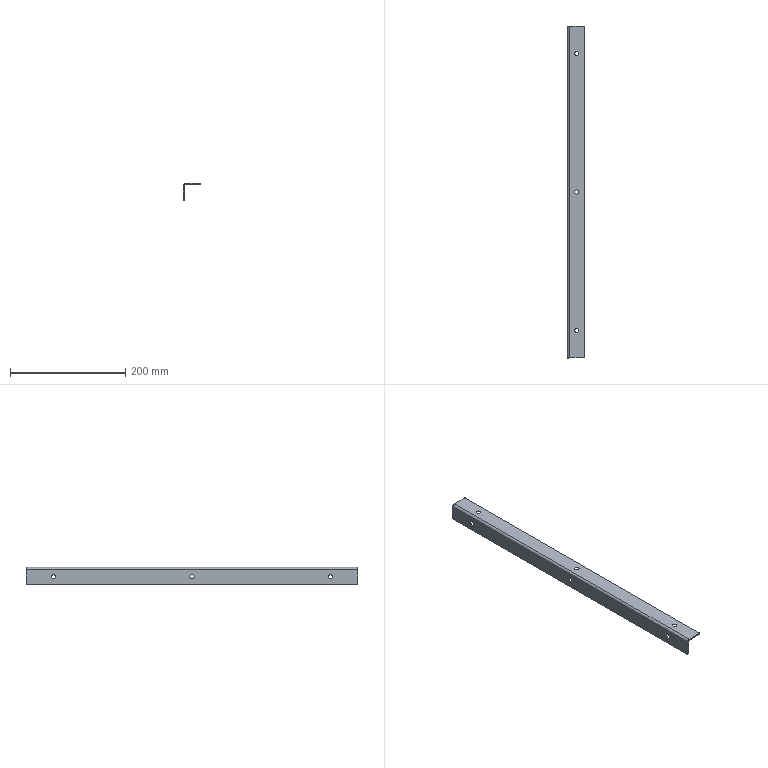Part | SolidWorks | features 3DProfileFeature 2, Fillet 2, HoleWzd 2, FlatPattern 1, ICE 1, LPattern 1, SMBaseFlange 1, SheetMetal 1 | 1 solid | 30 faces | box 30 x 575 x 30 mm | volume 64402 mm3 | cone 12 | plane 12 | cylinder 6 | commonest cylinder face diameters 4 x5 8 x1
STEP:
#1=CARTESIAN_POINT('',(-2.,-245.,-10.4));
#2=VERTEX_POINT('',#1);
#3=CARTESIAN_POINT('',(-2.,-245.,-17.6));
#4=VERTEX_POINT('',#3);
#5=CARTESIAN_POINT('',(-2.,-245.,-14.));
#6=DIRECTION('',(1.,0.,0.));
#7=DIRECTION('',(0.,0.,-1.));
#8=AXIS2_PLACEMENT_3D('',#5,#6,#7);
#9=CIRCLE('',#8,3.6);
#10=EDGE_CURVE('',#2,#4,#9,.T.);
#11=ORIENTED_EDGE('',*,*,#10,.F.);
#12=CARTESIAN_POINT('',(0.,-245.,-8.4));
#13=VERTEX_POINT('',#12);
#14=CARTESIAN_POINT('',(0.,-245.,-8.4));
#15=DIRECTION('',(0.7071,0.,0.7071));
#16=VECTOR('',#15,1000.);
#17=LINE('',#14,#16);
#18=EDGE_CURVE('',#2,#13,#17,.T.);
#19=ORIENTED_EDGE('',*,*,#18,.T.);
#20=CARTESIAN_POINT('',(0.,-245.,-19.6));
#21=VERTEX_POINT('',#20);
#22=CARTESIAN_POINT('',(0.,-245.,-14.));
#23=DIRECTION('',(1.,0.,0.));
#24=DIRECTION('',(0.,0.,-1.));
#25=AXIS2_PLACEMENT_3D('',#22,#23,#24);
#26=CIRCLE('',#25,5.6);
#27=EDGE_CURVE('',#13,#21,#26,.T.);
#28=ORIENTED_EDGE('',*,*,#27,.T.);
#29=CARTESIAN_POINT('',(0.,-245.,-19.6));
#30=DIRECTION('',(0.7071,0.,-0.7071));
#31=VECTOR('',#30,1000.);
#32=LINE('',#29,#31);
#33=EDGE_CURVE('',#4,#21,#32,.T.);
#34=ORIENTED_EDGE('',*,*,#33,.F.);
#35=EDGE_LOOP('',(#11,#19,#28,#34));
#36=FACE_OUTER_BOUND('',#35,.T.);
#37=CARTESIAN_POINT('',(0.,-245.,-14.));
#38=DIRECTION('',(1.,0.,0.));
#39=DIRECTION('',(0.,0.,-1.));
#40=AXIS2_PLACEMENT_3D('',#37,#38,#39);
#41=CONICAL_SURFACE('',#40,5.6,0.7854);
#42=ADVANCED_FACE('',(#36),#41,.F.);
#43=CARTESIAN_POINT('',(-2.,-5.,-10.4));
#44=VERTEX_POINT('',#43);
#45=CARTESIAN_POINT('',(-2.,-5.,-17.6));
#46=VERTEX_POINT('',#45);
#47=CARTESIAN_POINT('',(-2.,-5.,-14.));
#48=DIRECTION('',(1.,0.,0.));
#49=DIRECTION('',(0.,0.,-1.));
#50=AXIS2_PLACEMENT_3D('',#47,#48,#49);
#51=CIRCLE('',#50,3.6);
#52=EDGE_CURVE('',#44,#46,#51,.T.);
#53=ORIENTED_EDGE('',*,*,#52,.F.);
#54=CARTESIAN_POINT('',(0.,-5.,-8.4));
#55=VERTEX_POINT('',#54);
#56=CARTESIAN_POINT('',(0.,-5.,-8.4));
#57=DIRECTION('',(0.7071,0.,0.7071));
#58=VECTOR('',#57,1000.);
#59=LINE('',#56,#58);
#60=EDGE_CURVE('',#44,#55,#59,.T.);
#61=ORIENTED_EDGE('',*,*,#60,.T.);
#62=CARTESIAN_POINT('',(0.,-5.,-19.6));
#63=VERTEX_POINT('',#62);
#64=CARTESIAN_POINT('',(0.,-5.,-14.));
#65=DIRECTION('',(1.,0.,0.));
#66=DIRECTION('',(0.,0.,-1.));
#67=AXIS2_PLACEMENT_3D('',#64,#65,#66);
#68=CIRCLE('',#67,5.6);
#69=EDGE_CURVE('',#55,#63,#68,.T.);
#70=ORIENTED_EDGE('',*,*,#69,.T.);
#71=CARTESIAN_POINT('',(0.,-5.,-19.6));
#72=DIRECTION('',(0.7071,0.,-0.7071));
#73=VECTOR('',#72,1000.);
#74=LINE('',#71,#73);
#75=EDGE_CURVE('',#46,#63,#74,.T.);
#76=ORIENTED_EDGE('',*,*,#75,.F.);
#77=EDGE_LOOP('',(#53,#61,#70,#76));
#78=FACE_OUTER_BOUND('',#77,.T.);
#79=CARTESIAN_POINT('',(0.,-5.,-14.));
#80=DIRECTION('',(1.,0.,0.));
#81=DIRECTION('',(0.,0.,-1.));
#82=AXIS2_PLACEMENT_3D('',#79,#80,#81);
#83=CONICAL_SURFACE('',#82,5.6,0.7854);
#84=ADVANCED_FACE('',(#78),#83,.F.);
#85=CARTESIAN_POINT('',(17.6,-245.,2.));
#86=VERTEX_POINT('',#85);
#87=CARTESIAN_POINT('',(10.4,-245.,2.));
#88=VERTEX_POINT('',#87);
#89=CARTESIAN_POINT('',(14.,-245.,2.));
#90=DIRECTION('',(0.,0.,-1.));
#91=DIRECTION('',(-1.,0.,0.));
#92=AXIS2_PLACEMENT_3D('',#89,#90,#91);
#93=CIRCLE('',#92,3.6);
#94=EDGE_CURVE('',#86,#88,#93,.T.);
#95=ORIENTED_EDGE('',*,*,#94,.F.);
#96=CARTESIAN_POINT('',(19.6,-245.,0.));
#97=VERTEX_POINT('',#96);
#98=CARTESIAN_POINT('',(19.6,-245.,0.));
#99=DIRECTION('',(0.7071,0.,-0.7071));
#100=VECTOR('',#99,1000.);
#101=LINE('',#98,#100);
#102=EDGE_CURVE('',#86,#97,#101,.T.);
#103=ORIENTED_EDGE('',*,*,#102,.T.);
#104=CARTESIAN_POINT('',(8.4,-245.,0.));
#105=VERTEX_POINT('',#104);
#106=CARTESIAN_POINT('',(14.,-245.,0.));
#107=DIRECTION('',(0.,0.,-1.));
#108=DIRECTION('',(-1.,0.,0.));
#109=AXIS2_PLACEMENT_3D('',#106,#107,#108);
#110=CIRCLE('',#109,5.6);
#111=EDGE_CURVE('',#97,#105,#110,.T.);
#112=ORIENTED_EDGE('',*,*,#111,.T.);
#113=CARTESIAN_POINT('',(8.4,-245.,0.));
#114=DIRECTION('',(-0.7071,0.,-0.7071));
#115=VECTOR('',#114,1000.);
#116=LINE('',#113,#115);
#117=EDGE_CURVE('',#88,#105,#116,.T.);
#118=ORIENTED_EDGE('',*,*,#117,.F.);
#119=EDGE_LOOP('',(#95,#103,#112,#118));
#120=FACE_OUTER_BOUND('',#119,.T.);
#121=CARTESIAN_POINT('',(14.,-245.,0.));
#122=DIRECTION('',(0.,0.,-1.));
#123=DIRECTION('',(-1.,0.,0.));
#124=AXIS2_PLACEMENT_3D('',#121,#122,#123);
#125=CONICAL_SURFACE('',#124,5.6,0.7854);
#126=ADVANCED_FACE('',(#120),#125,.F.);
#127=CARTESIAN_POINT('',(17.6,-5.,2.));
#128=VERTEX_POINT('',#127);
#129=CARTESIAN_POINT('',(10.4,-5.,2.));
#130=VERTEX_POINT('',#129);
#131=CARTESIAN_POINT('',(14.,-5.,2.));
#132=DIRECTION('',(0.,0.,-1.));
#133=DIRECTION('',(-1.,0.,0.));
#134=AXIS2_PLACEMENT_3D('',#131,#132,#133);
#135=CIRCLE('',#134,3.6);
#136=EDGE_CURVE('',#128,#130,#135,.T.);
#137=ORIENTED_EDGE('',*,*,#136,.F.);
#138=CARTESIAN_POINT('',(19.6,-5.,0.));
#139=VERTEX_POINT('',#138);
#140=CARTESIAN_POINT('',(19.6,-5.,0.));
#141=DIRECTION('',(0.7071,0.,-0.7071));
#142=VECTOR('',#141,1000.);
#143=LINE('',#140,#142);
#144=EDGE_CURVE('',#128,#139,#143,.T.);
#145=ORIENTED_EDGE('',*,*,#144,.T.);
#146=CARTESIAN_POINT('',(8.4,-5.,0.));
#147=VERTEX_POINT('',#146);
#148=CARTESIAN_POINT('',(14.,-5.,0.));
#149=DIRECTION('',(0.,0.,-1.));
#150=DIRECTION('',(-1.,0.,0.));
#151=AXIS2_PLACEMENT_3D('',#148,#149,#150);
#152=CIRCLE('',#151,5.6);
#153=EDGE_CURVE('',#139,#147,#152,.T.);
#154=ORIENTED_EDGE('',*,*,#153,.T.);
#155=CARTESIAN_POINT('',(8.4,-5.,0.));
#156=DIRECTION('',(-0.7071,0.,-0.7071));
#157=VECTOR('',#156,1000.);
#158=LINE('',#155,#157);
#159=EDGE_CURVE('',#130,#147,#158,.T.);
#160=ORIENTED_EDGE('',*,*,#159,.F.);
#161=EDGE_LOOP('',(#137,#145,#154,#160));
#162=FACE_OUTER_BOUND('',#161,.T.);
#163=CARTESIAN_POINT('',(14.,-5.,0.));
#164=DIRECTION('',(0.,0.,-1.));
#165=DIRECTION('',(-1.,0.,0.));
#166=AXIS2_PLACEMENT_3D('',#163,#164,#165);
#167=CONICAL_SURFACE('',#166,5.6,0.7854);
#168=ADVANCED_FACE('',(#162),#167,.F.);
#169=CARTESIAN_POINT('',(-2.,235.,-10.4));
#170=VERTEX_POINT('',#169);
#171=CARTESIAN_POINT('',(-2.,235.,-17.6));
#172=VERTEX_POINT('',#171);
#173=CARTESIAN_POINT('',(-2.,235.,-14.));
#174=DIRECTION('',(1.,0.,0.));
#175=DIRECTION('',(0.,0.,-1.));
#176=AXIS2_PLACEMENT_3D('',#173,#174,#175);
#177=CIRCLE('',#176,3.6);
#178=EDGE_CURVE('',#170,#172,#177,.T.);
#179=ORIENTED_EDGE('',*,*,#178,.F.);
#180=CARTESIAN_POINT('',(0.,235.,-8.4));
#181=VERTEX_POINT('',#180);
#182=CARTESIAN_POINT('',(0.,235.,-8.4));
#183=DIRECTION('',(0.7071,0.,0.7071));
#184=VECTOR('',#183,1000.);
#185=LINE('',#182,#184);
#186=EDGE_CURVE('',#170,#181,#185,.T.);
#187=ORIENTED_EDGE('',*,*,#186,.T.);
#188=CARTESIAN_POINT('',(0.,235.,-19.6));
#189=VERTEX_POINT('',#188);
#190=CARTESIAN_POINT('',(0.,235.,-14.));
#191=DIRECTION('',(1.,0.,0.));
#192=DIRECTION('',(0.,0.,-1.));
#193=AXIS2_PLACEMENT_3D('',#190,#191,#192);
#194=CIRCLE('',#193,5.6);
#195=EDGE_CURVE('',#181,#189,#194,.T.);
#196=ORIENTED_EDGE('',*,*,#195,.T.);
#197=CARTESIAN_POINT('',(0.,235.,-19.6));
#198=DIRECTION('',(0.7071,0.,-0.7071));
#199=VECTOR('',#198,1000.);
#200=LINE('',#197,#199);
#201=EDGE_CURVE('',#172,#189,#200,.T.);
#202=ORIENTED_EDGE('',*,*,#201,.F.);
#203=EDGE_LOOP('',(#179,#187,#196,#202));
#204=FACE_OUTER_BOUND('',#203,.T.);
#205=CARTESIAN_POINT('',(0.,235.,-14.));
#206=DIRECTION('',(1.,0.,0.));
#207=DIRECTION('',(0.,0.,-1.));
#208=AXIS2_PLACEMENT_3D('',#205,#206,#207);
#209=CONICAL_SURFACE('',#208,5.6,0.7854);
#210=ADVANCED_FACE('',(#204),#209,.F.);
#211=CARTESIAN_POINT('',(17.6,235.,2.));
#212=VERTEX_POINT('',#211);
#213=CARTESIAN_POINT('',(10.4,235.,2.));
#214=VERTEX_POINT('',#213);
#215=CARTESIAN_POINT('',(14.,235.,2.));
#216=DIRECTION('',(0.,0.,-1.));
#217=DIRECTION('',(-1.,0.,0.));
#218=AXIS2_PLACEMENT_3D('',#215,#216,#217);
#219=CIRCLE('',#218,3.6);
#220=EDGE_CURVE('',#212,#214,#219,.T.);
#221=ORIENTED_EDGE('',*,*,#220,.F.);
#222=CARTESIAN_POINT('',(19.6,235.,0.));
#223=VERTEX_POINT('',#222);
#224=CARTESIAN_POINT('',(19.6,235.,0.));
#225=DIRECTION('',(0.7071,0.,-0.7071));
#226=VECTOR('',#225,1000.);
#227=LINE('',#224,#226);
#228=EDGE_CURVE('',#212,#223,#227,.T.);
#229=ORIENTED_EDGE('',*,*,#228,.T.);
#230=CARTESIAN_POINT('',(8.4,235.,0.));
#231=VERTEX_POINT('',#230);
#232=CARTESIAN_POINT('',(14.,235.,0.));
#233=DIRECTION('',(0.,0.,-1.));
#234=DIRECTION('',(-1.,0.,0.));
#235=AXIS2_PLACEMENT_3D('',#232,#233,#234);
#236=CIRCLE('',#235,5.6);
#237=EDGE_CURVE('',#223,#231,#236,.T.);
#238=ORIENTED_EDGE('',*,*,#237,.T.);
#239=CARTESIAN_POINT('',(8.4,235.,0.));
#240=DIRECTION('',(-0.7071,0.,-0.7071));
#241=VECTOR('',#240,1000.);
#242=LINE('',#239,#241);
#243=EDGE_CURVE('',#214,#231,#242,.T.);
#244=ORIENTED_EDGE('',*,*,#243,.F.);
#245=EDGE_LOOP('',(#221,#229,#238,#244));
#246=FACE_OUTER_BOUND('',#245,.T.);
#247=CARTESIAN_POINT('',(14.,235.,0.));
#248=DIRECTION('',(0.,0.,-1.));
#249=DIRECTION('',(-1.,0.,0.));
#250=AXIS2_PLACEMENT_3D('',#247,#248,#249);
#251=CONICAL_SURFACE('',#250,5.6,0.7854);
#252=ADVANCED_FACE('',(#246),#251,.F.);
#253=CARTESIAN_POINT('',(0.,282.5,-26.));
#254=VERTEX_POINT('',#253);
#255=CARTESIAN_POINT('',(0.,282.5,-2.));
#256=VERTEX_POINT('',#255);
#257=CARTESIAN_POINT('',(0.,282.5,-28.));
#258=DIRECTION('',(0.,0.,1.));
#259=VECTOR('',#258,1000.);
#260=LINE('',#257,#259);
#261=EDGE_CURVE('',#254,#256,#260,.T.);
#262=ORIENTED_EDGE('',*,*,#261,.F.);
#263=CARTESIAN_POINT('',(-2.,282.5,-26.));
#264=VERTEX_POINT('',#263);
#265=CARTESIAN_POINT('',(28.,282.5,-26.));
#266=DIRECTION('',(-1.,0.,0.));
#267=VECTOR('',#266,1000.);
#268=LINE('',#265,#267);
#269=EDGE_CURVE('',#254,#264,#268,.T.);
#270=ORIENTED_EDGE('',*,*,#269,.T.);
#271=CARTESIAN_POINT('',(-2.,282.5,-2.));
#272=VERTEX_POINT('',#271);
#273=CARTESIAN_POINT('',(-2.,282.5,18.726));
#274=DIRECTION('',(0.,0.,-1.));
#275=VECTOR('',#274,1000.);
#276=LINE('',#273,#275);
#277=EDGE_CURVE('',#272,#264,#276,.T.);
#278=ORIENTED_EDGE('',*,*,#277,.F.);
#279=CARTESIAN_POINT('',(-2.,282.5,-2.));
#280=DIRECTION('',(1.,0.,0.));
#281=VECTOR('',#280,1000.);
#282=LINE('',#279,#281);
#283=EDGE_CURVE('',#272,#256,#282,.T.);
#284=ORIENTED_EDGE('',*,*,#283,.T.);
#285=EDGE_LOOP('',(#262,#270,#278,#284));
#286=FACE_OUTER_BOUND('',#285,.T.);
#287=CARTESIAN_POINT('',(28.,282.5,18.726));
#288=DIRECTION('',(0.,1.,0.));
#289=DIRECTION('',(0.,0.,1.));
#290=AXIS2_PLACEMENT_3D('',#287,#288,#289);
#291=PLANE('',#290);
#292=ADVANCED_FACE('',(#286),#291,.T.);
#293=CARTESIAN_POINT('',(2.,282.5,2.));
#294=VERTEX_POINT('',#293);
#295=CARTESIAN_POINT('',(26.,282.5,2.));
#296=VERTEX_POINT('',#295);
#297=CARTESIAN_POINT('',(0.,282.5,2.));
#298=DIRECTION('',(1.,0.,0.));
#299=VECTOR('',#298,1000.);
#300=LINE('',#297,#299);
#301=EDGE_CURVE('',#294,#296,#300,.T.);
#302=ORIENTED_EDGE('',*,*,#301,.T.);
#303=CARTESIAN_POINT('',(26.,282.5,0.));
#304=VERTEX_POINT('',#303);
#305=CARTESIAN_POINT('',(26.,282.5,18.726));
#306=DIRECTION('',(0.,0.,-1.));
#307=VECTOR('',#306,1000.);
#308=LINE('',#305,#307);
#309=EDGE_CURVE('',#296,#304,#308,.T.);
#310=ORIENTED_EDGE('',*,*,#309,.T.);
#311=CARTESIAN_POINT('',(2.,282.5,0.));
#312=VERTEX_POINT('',#311);
#313=CARTESIAN_POINT('',(0.,282.5,0.));
#314=DIRECTION('',(1.,0.,0.));
#315=VECTOR('',#314,1000.);
#316=LINE('',#313,#315);
#317=EDGE_CURVE('',#312,#304,#316,.T.);
#318=ORIENTED_EDGE('',*,*,#317,.F.);
#319=CARTESIAN_POINT('',(2.,282.5,0.));
#320=DIRECTION('',(0.,0.,1.));
#321=VECTOR('',#320,1000.);
#322=LINE('',#319,#321);
#323=EDGE_CURVE('',#312,#294,#322,.T.);
#324=ORIENTED_EDGE('',*,*,#323,.T.);
#325=EDGE_LOOP('',(#302,#310,#318,#324));
#326=FACE_OUTER_BOUND('',#325,.T.);
#327=CARTESIAN_POINT('',(28.,282.5,18.726));
#328=DIRECTION('',(0.,1.,0.));
#329=DIRECTION('',(0.,0.,1.));
#330=AXIS2_PLACEMENT_3D('',#327,#328,#329);
#331=PLANE('',#330);
#332=ADVANCED_FACE('',(#326),#331,.T.);
#333=CARTESIAN_POINT('',(14.,235.,2.));
#334=DIRECTION('',(0.,0.,-1.));
#335=DIRECTION('',(-1.,0.,0.));
#336=AXIS2_PLACEMENT_3D('',#333,#334,#335);
#337=CIRCLE('',#336,3.6);
#338=EDGE_CURVE('',#214,#212,#337,.T.);
#339=ORIENTED_EDGE('',*,*,#338,.T.);
#340=ORIENTED_EDGE('',*,*,#220,.T.);
#341=EDGE_LOOP('',(#339,#340));
#342=FACE_BOUND('',#341,.T.);
#343=CARTESIAN_POINT('',(14.,-5.,2.));
#344=DIRECTION('',(0.,0.,-1.));
#345=DIRECTION('',(-1.,0.,0.));
#346=AXIS2_PLACEMENT_3D('',#343,#344,#345);
#347=CIRCLE('',#346,3.6);
#348=EDGE_CURVE('',#130,#128,#347,.T.);
#349=ORIENTED_EDGE('',*,*,#348,.T.);
#350=ORIENTED_EDGE('',*,*,#136,.T.);
#351=EDGE_LOOP('',(#349,#350));
#352=FACE_BOUND('',#351,.T.);
#353=CARTESIAN_POINT('',(14.,-245.,2.));
#354=DIRECTION('',(0.,0.,-1.));
#355=DIRECTION('',(-1.,0.,0.));
#356=AXIS2_PLACEMENT_3D('',#353,#354,#355);
#357=CIRCLE('',#356,3.6);
#358=EDGE_CURVE('',#88,#86,#357,.T.);
#359=ORIENTED_EDGE('',*,*,#358,.T.);
#360=ORIENTED_EDGE('',*,*,#94,.T.);
#361=EDGE_LOOP('',(#359,#360));
#362=FACE_BOUND('',#361,.T.);
#363=CARTESIAN_POINT('',(28.,280.5,2.));
#364=VERTEX_POINT('',#363);
#365=CARTESIAN_POINT('',(28.,-290.5,2.));
#366=VERTEX_POINT('',#365);
#367=CARTESIAN_POINT('',(28.,292.5,2.));
#368=DIRECTION('',(0.,-1.,0.));
#369=VECTOR('',#368,1000.);
#370=LINE('',#367,#369);
#371=EDGE_CURVE('',#364,#366,#370,.T.);
#372=ORIENTED_EDGE('',*,*,#371,.F.);
#373=CARTESIAN_POINT('',(26.,280.5,2.));
#374=DIRECTION('',(0.,0.,1.));
#375=DIRECTION('',(-1.,0.,0.));
#376=AXIS2_PLACEMENT_3D('',#373,#374,#375);
#377=CIRCLE('',#376,2.);
#378=EDGE_CURVE('',#364,#296,#377,.T.);
#379=ORIENTED_EDGE('',*,*,#378,.T.);
#380=ORIENTED_EDGE('',*,*,#301,.F.);
#381=CARTESIAN_POINT('',(2.,-292.5,2.));
#382=VERTEX_POINT('',#381);
#383=CARTESIAN_POINT('',(2.,292.5,2.));
#384=DIRECTION('',(0.,-1.,0.));
#385=VECTOR('',#384,1000.);
#386=LINE('',#383,#385);
#387=EDGE_CURVE('',#294,#382,#386,.T.);
#388=ORIENTED_EDGE('',*,*,#387,.T.);
#389=CARTESIAN_POINT('',(26.,-292.5,2.));
#390=VERTEX_POINT('',#389);
#391=CARTESIAN_POINT('',(0.,-292.5,2.));
#392=DIRECTION('',(1.,0.,0.));
#393=VECTOR('',#392,1000.);
#394=LINE('',#391,#393);
#395=EDGE_CURVE('',#382,#390,#394,.T.);
#396=ORIENTED_EDGE('',*,*,#395,.T.);
#397=CARTESIAN_POINT('',(26.,-290.5,2.));
#398=DIRECTION('',(0.,0.,1.));
#399=DIRECTION('',(-1.,0.,0.));
#400=AXIS2_PLACEMENT_3D('',#397,#398,#399);
#401=CIRCLE('',#400,2.);
#402=EDGE_CURVE('',#390,#366,#401,.T.);
#403=ORIENTED_EDGE('',*,*,#402,.T.);
#404=EDGE_LOOP('',(#372,#379,#380,#388,#396,#403));
#405=FACE_OUTER_BOUND('',#404,.T.);
#406=CARTESIAN_POINT('',(0.,292.5,2.));
#407=DIRECTION('',(0.,0.,-1.));
#408=DIRECTION('',(-1.,0.,0.));
#409=AXIS2_PLACEMENT_3D('',#406,#407,#408);
#410=PLANE('',#409);
#411=ADVANCED_FACE('',(#342,#352,#362,#405),#410,.F.);
#412=CARTESIAN_POINT('',(28.,280.5,0.));
#413=VERTEX_POINT('',#412);
#414=CARTESIAN_POINT('',(28.,-290.5,0.));
#415=VERTEX_POINT('',#414);
#416=CARTESIAN_POINT('',(28.,292.5,0.));
#417=DIRECTION('',(0.,-1.,0.));
#418=VECTOR('',#417,1000.);
#419=LINE('',#416,#418);
#420=EDGE_CURVE('',#413,#415,#419,.T.);
#421=ORIENTED_EDGE('',*,*,#420,.F.);
#422=CARTESIAN_POINT('',(28.,280.5,0.));
#423=DIRECTION('',(0.,0.,1.));
#424=VECTOR('',#423,1000.);
#425=LINE('',#422,#424);
#426=EDGE_CURVE('',#413,#364,#425,.T.);
#427=ORIENTED_EDGE('',*,*,#426,.T.);
#428=ORIENTED_EDGE('',*,*,#371,.T.);
#429=CARTESIAN_POINT('',(28.,-290.5,0.));
#430=DIRECTION('',(0.,0.,-1.));
#431=VECTOR('',#430,1000.);
#432=LINE('',#429,#431);
#433=EDGE_CURVE('',#366,#415,#432,.T.);
#434=ORIENTED_EDGE('',*,*,#433,.T.);
#435=EDGE_LOOP('',(#421,#427,#428,#434));
#436=FACE_OUTER_BOUND('',#435,.T.);
#437=CARTESIAN_POINT('',(28.,292.5,0.));
#438=DIRECTION('',(1.,0.,0.));
#439=DIRECTION('',(0.,0.,-1.));
#440=AXIS2_PLACEMENT_3D('',#437,#438,#439);
#441=PLANE('',#440);
#442=ADVANCED_FACE('',(#436),#441,.T.);
#443=CARTESIAN_POINT('',(14.,-245.,0.));
#444=DIRECTION('',(0.,0.,-1.));
#445=DIRECTION('',(-1.,0.,0.));
#446=AXIS2_PLACEMENT_3D('',#443,#444,#445);
#447=CIRCLE('',#446,5.6);
#448=EDGE_CURVE('',#105,#97,#447,.T.);
#449=ORIENTED_EDGE('',*,*,#448,.F.);
#450=ORIENTED_EDGE('',*,*,#111,.F.);
#451=EDGE_LOOP('',(#449,#450));
#452=FACE_BOUND('',#451,.T.);
#453=CARTESIAN_POINT('',(14.,-5.,0.));
#454=DIRECTION('',(0.,0.,-1.));
#455=DIRECTION('',(-1.,0.,0.));
#456=AXIS2_PLACEMENT_3D('',#453,#454,#455);
#457=CIRCLE('',#456,5.6);
#458=EDGE_CURVE('',#147,#139,#457,.T.);
#459=ORIENTED_EDGE('',*,*,#458,.F.);
#460=ORIENTED_EDGE('',*,*,#153,.F.);
#461=EDGE_LOOP('',(#459,#460));
#462=FACE_BOUND('',#461,.T.);
#463=CARTESIAN_POINT('',(14.,235.,0.));
#464=DIRECTION('',(0.,0.,-1.));
#465=DIRECTION('',(-1.,0.,0.));
#466=AXIS2_PLACEMENT_3D('',#463,#464,#465);
#467=CIRCLE('',#466,5.6);
#468=EDGE_CURVE('',#231,#223,#467,.T.);
#469=ORIENTED_EDGE('',*,*,#468,.F.);
#470=ORIENTED_EDGE('',*,*,#237,.F.);
#471=EDGE_LOOP('',(#469,#470));
#472=FACE_BOUND('',#471,.T.);
#473=ORIENTED_EDGE('',*,*,#317,.T.);
#474=CARTESIAN_POINT('',(26.,280.5,0.));
#475=DIRECTION('',(0.,0.,-1.));
#476=DIRECTION('',(-1.,0.,0.));
#477=AXIS2_PLACEMENT_3D('',#474,#475,#476);
#478=CIRCLE('',#477,2.);
#479=EDGE_CURVE('',#304,#413,#478,.T.);
#480=ORIENTED_EDGE('',*,*,#479,.T.);
#481=ORIENTED_EDGE('',*,*,#420,.T.);
#482=CARTESIAN_POINT('',(26.,-292.5,0.));
#483=VERTEX_POINT('',#482);
#484=CARTESIAN_POINT('',(26.,-290.5,0.));
#485=DIRECTION('',(0.,0.,-1.));
#486=DIRECTION('',(-1.,0.,0.));
#487=AXIS2_PLACEMENT_3D('',#484,#485,#486);
#488=CIRCLE('',#487,2.);
#489=EDGE_CURVE('',#415,#483,#488,.T.);
#490=ORIENTED_EDGE('',*,*,#489,.T.);
#491=CARTESIAN_POINT('',(2.,-292.5,0.));
#492=VERTEX_POINT('',#491);
#493=CARTESIAN_POINT('',(0.,-292.5,0.));
#494=DIRECTION('',(1.,0.,0.));
#495=VECTOR('',#494,1000.);
#496=LINE('',#493,#495);
#497=EDGE_CURVE('',#492,#483,#496,.T.);
#498=ORIENTED_EDGE('',*,*,#497,.F.);
#499=CARTESIAN_POINT('',(2.,292.5,0.));
#500=DIRECTION('',(0.,-1.,0.));
#501=VECTOR('',#500,1000.);
#502=LINE('',#499,#501);
#503=EDGE_CURVE('',#312,#492,#502,.T.);
#504=ORIENTED_EDGE('',*,*,#503,.F.);
#505=EDGE_LOOP('',(#473,#480,#481,#490,#498,#504));
#506=FACE_OUTER_BOUND('',#505,.T.);
#507=CARTESIAN_POINT('',(0.,292.5,0.));
#508=DIRECTION('',(0.,0.,-1.));
#509=DIRECTION('',(-1.,0.,0.));
#510=AXIS2_PLACEMENT_3D('',#507,#508,#509);
#511=PLANE('',#510);
#512=ADVANCED_FACE('',(#452,#462,#472,#506),#511,.T.);
#513=CARTESIAN_POINT('',(0.,-292.5,-2.));
#514=VERTEX_POINT('',#513);
#515=CARTESIAN_POINT('',(0.,292.5,-2.));
#516=DIRECTION('',(0.,-1.,0.));
#517=VECTOR('',#516,1000.);
#518=LINE('',#515,#517);
#519=EDGE_CURVE('',#256,#514,#518,.T.);
#520=ORIENTED_EDGE('',*,*,#519,.F.);
#521=CARTESIAN_POINT('',(2.,282.5,-2.));
#522=DIRECTION('',(0.,1.,0.));
#523=DIRECTION('',(0.,0.,1.));
#524=AXIS2_PLACEMENT_3D('',#521,#522,#523);
#525=CIRCLE('',#524,2.);
#526=EDGE_CURVE('',#256,#312,#525,.T.);
#527=ORIENTED_EDGE('',*,*,#526,.T.);
#528=ORIENTED_EDGE('',*,*,#503,.T.);
#529=CARTESIAN_POINT('',(2.,-292.5,-2.));
#530=DIRECTION('',(0.,1.,0.));
#531=DIRECTION('',(0.,0.,-1.));
#532=AXIS2_PLACEMENT_3D('',#529,#530,#531);
#533=CIRCLE('',#532,2.);
#534=EDGE_CURVE('',#514,#492,#533,.T.);
#535=ORIENTED_EDGE('',*,*,#534,.F.);
#536=EDGE_LOOP('',(#520,#527,#528,#535));
#537=FACE_OUTER_BOUND('',#536,.T.);
#538=CARTESIAN_POINT('',(2.,292.5,-2.));
#539=DIRECTION('',(0.,-1.,0.));
#540=DIRECTION('',(0.,0.,-1.));
#541=AXIS2_PLACEMENT_3D('',#538,#539,#540);
#542=CYLINDRICAL_SURFACE('',#541,2.);
#543=ADVANCED_FACE('',(#537),#542,.F.);
#544=CARTESIAN_POINT('',(0.,-245.,-14.));
#545=DIRECTION('',(1.,0.,0.));
#546=DIRECTION('',(0.,0.,-1.));
#547=AXIS2_PLACEMENT_3D('',#544,#545,#546);
#548=CIRCLE('',#547,5.6);
#549=EDGE_CURVE('',#21,#13,#548,.T.);
#550=ORIENTED_EDGE('',*,*,#549,.F.);
#551=ORIENTED_EDGE('',*,*,#27,.F.);
#552=EDGE_LOOP('',(#550,#551));
#553=FACE_BOUND('',#552,.T.);
#554=CARTESIAN_POINT('',(0.,-5.,-14.));
#555=DIRECTION('',(1.,0.,0.));
#556=DIRECTION('',(0.,0.,-1.));
#557=AXIS2_PLACEMENT_3D('',#554,#555,#556);
#558=CIRCLE('',#557,5.6);
#559=EDGE_CURVE('',#63,#55,#558,.T.);
#560=ORIENTED_EDGE('',*,*,#559,.F.);
#561=ORIENTED_EDGE('',*,*,#69,.F.);
#562=EDGE_LOOP('',(#560,#561));
#563=FACE_BOUND('',#562,.T.);
#564=CARTESIAN_POINT('',(0.,235.,-14.));
#565=DIRECTION('',(1.,0.,0.));
#566=DIRECTION('',(0.,0.,-1.));
#567=AXIS2_PLACEMENT_3D('',#564,#565,#566);
#568=CIRCLE('',#567,5.6);
#569=EDGE_CURVE('',#189,#181,#568,.T.);
#570=ORIENTED_EDGE('',*,*,#569,.F.);
#571=ORIENTED_EDGE('',*,*,#195,.F.);
#572=EDGE_LOOP('',(#570,#571));
#573=FACE_BOUND('',#572,.T.);
#574=CARTESIAN_POINT('',(0.,280.5,-28.));
#575=VERTEX_POINT('',#574);
#576=CARTESIAN_POINT('',(0.,-290.5,-28.));
#577=VERTEX_POINT('',#576);
#578=CARTESIAN_POINT('',(0.,292.5,-28.));
#579=DIRECTION('',(0.,-1.,0.));
#580=VECTOR('',#579,1000.);
#581=LINE('',#578,#580);
#582=EDGE_CURVE('',#575,#577,#581,.T.);
#583=ORIENTED_EDGE('',*,*,#582,.F.);
#584=CARTESIAN_POINT('',(0.,280.5,-26.));
#585=DIRECTION('',(1.,0.,0.));
#586=DIRECTION('',(0.,0.,-1.));
#587=AXIS2_PLACEMENT_3D('',#584,#585,#586);
#588=CIRCLE('',#587,2.);
#589=EDGE_CURVE('',#575,#254,#588,.T.);
#590=ORIENTED_EDGE('',*,*,#589,.T.);
#591=ORIENTED_EDGE('',*,*,#261,.T.);
#592=ORIENTED_EDGE('',*,*,#519,.T.);
#593=CARTESIAN_POINT('',(0.,-292.5,-26.));
#594=VERTEX_POINT('',#593);
#595=CARTESIAN_POINT('',(0.,-292.5,-28.));
#596=DIRECTION('',(0.,0.,1.));
#597=VECTOR('',#596,1000.);
#598=LINE('',#595,#597);
#599=EDGE_CURVE('',#594,#514,#598,.T.);
#600=ORIENTED_EDGE('',*,*,#599,.F.);
#601=CARTESIAN_POINT('',(0.,-290.5,-26.));
#602=DIRECTION('',(1.,0.,0.));
#603=DIRECTION('',(0.,0.,-1.));
#604=AXIS2_PLACEMENT_3D('',#601,#602,#603);
#605=CIRCLE('',#604,2.);
#606=EDGE_CURVE('',#594,#577,#605,.T.);
#607=ORIENTED_EDGE('',*,*,#606,.T.);
#608=EDGE_LOOP('',(#583,#590,#591,#592,#600,#607));
#609=FACE_OUTER_BOUND('',#608,.T.);
#610=CARTESIAN_POINT('',(0.,292.5,-28.));
#611=DIRECTION('',(1.,0.,0.));
#612=DIRECTION('',(0.,0.,-1.));
#613=AXIS2_PLACEMENT_3D('',#610,#611,#612);
#614=PLANE('',#613);
#615=ADVANCED_FACE('',(#553,#563,#573,#609),#614,.T.);
#616=CARTESIAN_POINT('',(-2.,280.5,-28.));
#617=VERTEX_POINT('',#616);
#618=CARTESIAN_POINT('',(-2.,-290.5,-28.));
#619=VERTEX_POINT('',#618);
#620=CARTESIAN_POINT('',(-2.,292.5,-28.));
#621=DIRECTION('',(0.,-1.,0.));
#622=VECTOR('',#621,1000.);
#623=LINE('',#620,#622);
#624=EDGE_CURVE('',#617,#619,#623,.T.);
#625=ORIENTED_EDGE('',*,*,#624,.F.);
#626=CARTESIAN_POINT('',(-2.,280.5,-28.));
#627=DIRECTION('',(1.,0.,0.));
#628=VECTOR('',#627,1000.);
#629=LINE('',#626,#628);
#630=EDGE_CURVE('',#617,#575,#629,.T.);
#631=ORIENTED_EDGE('',*,*,#630,.T.);
#632=ORIENTED_EDGE('',*,*,#582,.T.);
#633=CARTESIAN_POINT('',(-2.,-290.5,-28.));
#634=DIRECTION('',(-1.,0.,0.));
#635=VECTOR('',#634,1000.);
#636=LINE('',#633,#635);
#637=EDGE_CURVE('',#577,#619,#636,.T.);
#638=ORIENTED_EDGE('',*,*,#637,.T.);
#639=EDGE_LOOP('',(#625,#631,#632,#638));
#640=FACE_OUTER_BOUND('',#639,.T.);
#641=CARTESIAN_POINT('',(-2.,292.5,-28.));
#642=DIRECTION('',(0.,0.,-1.));
#643=DIRECTION('',(-1.,0.,0.));
#644=AXIS2_PLACEMENT_3D('',#641,#642,#643);
#645=PLANE('',#644);
#646=ADVANCED_FACE('',(#640),#645,.T.);
#647=CARTESIAN_POINT('',(-2.,235.,-14.));
#648=DIRECTION('',(1.,0.,0.));
#649=DIRECTION('',(0.,0.,-1.));
#650=AXIS2_PLACEMENT_3D('',#647,#648,#649);
#651=CIRCLE('',#650,3.6);
#652=EDGE_CURVE('',#172,#170,#651,.T.);
#653=ORIENTED_EDGE('',*,*,#652,.T.);
#654=ORIENTED_EDGE('',*,*,#178,.T.);
#655=EDGE_LOOP('',(#653,#654));
#656=FACE_BOUND('',#655,.T.);
#657=CARTESIAN_POINT('',(-2.,-5.,-14.));
#658=DIRECTION('',(1.,0.,0.));
#659=DIRECTION('',(0.,0.,-1.));
#660=AXIS2_PLACEMENT_3D('',#657,#658,#659);
#661=CIRCLE('',#660,3.6);
#662=EDGE_CURVE('',#46,#44,#661,.T.);
#663=ORIENTED_EDGE('',*,*,#662,.T.);
#664=ORIENTED_EDGE('',*,*,#52,.T.);
#665=EDGE_LOOP('',(#663,#664));
#666=FACE_BOUND('',#665,.T.);
#667=CARTESIAN_POINT('',(-2.,-245.,-14.));
#668=DIRECTION('',(1.,0.,0.));
#669=DIRECTION('',(0.,0.,-1.));
#670=AXIS2_PLACEMENT_3D('',#667,#668,#669);
#671=CIRCLE('',#670,3.6);
#672=EDGE_CURVE('',#4,#2,#671,.T.);
#673=ORIENTED_EDGE('',*,*,#672,.T.);
#674=ORIENTED_EDGE('',*,*,#10,.T.);
#675=EDGE_LOOP('',(#673,#674));
#676=FACE_BOUND('',#675,.T.);
#677=ORIENTED_EDGE('',*,*,#277,.T.);
#678=CARTESIAN_POINT('',(-2.,280.5,-26.));
#679=DIRECTION('',(-1.,0.,0.));
#680=DIRECTION('',(0.,0.,-1.));
#681=AXIS2_PLACEMENT_3D('',#678,#679,#680);
#682=CIRCLE('',#681,2.);
#683=EDGE_CURVE('',#264,#617,#682,.T.);
#684=ORIENTED_EDGE('',*,*,#683,.T.);
#685=ORIENTED_EDGE('',*,*,#624,.T.);
#686=CARTESIAN_POINT('',(-2.,-292.5,-26.));
#687=VERTEX_POINT('',#686);
#688=CARTESIAN_POINT('',(-2.,-290.5,-26.));
#689=DIRECTION('',(-1.,0.,0.));
#690=DIRECTION('',(0.,0.,-1.));
#691=AXIS2_PLACEMENT_3D('',#688,#689,#690);
#692=CIRCLE('',#691,2.);
#693=EDGE_CURVE('',#619,#687,#692,.T.);
#694=ORIENTED_EDGE('',*,*,#693,.T.);
#695=CARTESIAN_POINT('',(-2.,-292.5,-2.));
#696=VERTEX_POINT('',#695);
#697=CARTESIAN_POINT('',(-2.,-292.5,-28.));
#698=DIRECTION('',(0.,0.,1.));
#699=VECTOR('',#698,1000.);
#700=LINE('',#697,#699);
#701=EDGE_CURVE('',#687,#696,#700,.T.);
#702=ORIENTED_EDGE('',*,*,#701,.T.);
#703=CARTESIAN_POINT('',(-2.,292.5,-2.));
#704=DIRECTION('',(0.,-1.,0.));
#705=VECTOR('',#704,1000.);
#706=LINE('',#703,#705);
#707=EDGE_CURVE('',#272,#696,#706,.T.);
#708=ORIENTED_EDGE('',*,*,#707,.F.);
#709=EDGE_LOOP('',(#677,#684,#685,#694,#702,#708));
#710=FACE_OUTER_BOUND('',#709,.T.);
#711=CARTESIAN_POINT('',(-2.,292.5,-28.));
#712=DIRECTION('',(1.,0.,0.));
#713=DIRECTION('',(0.,0.,-1.));
#714=AXIS2_PLACEMENT_3D('',#711,#712,#713);
#715=PLANE('',#714);
#716=ADVANCED_FACE('',(#656,#666,#676,#710),#715,.F.);
#717=CARTESIAN_POINT('',(2.,282.5,-2.));
#718=DIRECTION('',(0.,1.,0.));
#719=DIRECTION('',(0.,0.,1.));
#720=AXIS2_PLACEMENT_3D('',#717,#718,#719);
#721=CIRCLE('',#720,4.);
#722=EDGE_CURVE('',#272,#294,#721,.T.);
#723=ORIENTED_EDGE('',*,*,#722,.F.);
#724=ORIENTED_EDGE('',*,*,#707,.T.);
#725=CARTESIAN_POINT('',(2.,-292.5,-2.));
#726=DIRECTION('',(0.,1.,0.));
#727=DIRECTION('',(1.,0.,0.));
#728=AXIS2_PLACEMENT_3D('',#725,#726,#727);
#729=CIRCLE('',#728,4.);
#730=EDGE_CURVE('',#696,#382,#729,.T.);
#731=ORIENTED_EDGE('',*,*,#730,.T.);
#732=ORIENTED_EDGE('',*,*,#387,.F.);
#733=EDGE_LOOP('',(#723,#724,#731,#732));
#734=FACE_OUTER_BOUND('',#733,.T.);
#735=CARTESIAN_POINT('',(2.,292.5,-2.));
#736=DIRECTION('',(0.,-1.,0.));
#737=DIRECTION('',(0.,0.,-1.));
#738=AXIS2_PLACEMENT_3D('',#735,#736,#737);
#739=CYLINDRICAL_SURFACE('',#738,4.);
#740=ADVANCED_FACE('',(#734),#739,.T.);
#741=CARTESIAN_POINT('',(0.,-292.5,-2.));
#742=DIRECTION('',(-1.,0.,0.));
#743=VECTOR('',#742,1000.);
#744=LINE('',#741,#743);
#745=EDGE_CURVE('',#514,#696,#744,.T.);
#746=ORIENTED_EDGE('',*,*,#745,.F.);
#747=ORIENTED_EDGE('',*,*,#534,.T.);
#748=CARTESIAN_POINT('',(2.,-292.5,2.));
#749=DIRECTION('',(0.,0.,-1.));
#750=VECTOR('',#749,1000.);
#751=LINE('',#748,#750);
#752=EDGE_CURVE('',#382,#492,#751,.T.);
#753=ORIENTED_EDGE('',*,*,#752,.F.);
#754=ORIENTED_EDGE('',*,*,#730,.F.);
#755=EDGE_LOOP('',(#746,#747,#753,#754));
#756=FACE_OUTER_BOUND('',#755,.T.);
#757=CARTESIAN_POINT('',(0.,-292.5,-2.));
#758=DIRECTION('',(0.,-1.,0.));
#759=DIRECTION('',(0.,0.,-1.));
#760=AXIS2_PLACEMENT_3D('',#757,#758,#759);
#761=PLANE('',#760);
#762=ADVANCED_FACE('',(#756),#761,.T.);
#763=ORIENTED_EDGE('',*,*,#701,.F.);
#764=CARTESIAN_POINT('',(2.,-292.5,-26.));
#765=DIRECTION('',(1.,0.,0.));
#766=VECTOR('',#765,1000.);
#767=LINE('',#764,#766);
#768=EDGE_CURVE('',#687,#594,#767,.T.);
#769=ORIENTED_EDGE('',*,*,#768,.T.);
#770=ORIENTED_EDGE('',*,*,#599,.T.);
#771=ORIENTED_EDGE('',*,*,#745,.T.);
#772=EDGE_LOOP('',(#763,#769,#770,#771));
#773=FACE_OUTER_BOUND('',#772,.T.);
#774=CARTESIAN_POINT('',(2.,-292.5,2.));
#775=DIRECTION('',(0.,-1.,0.));
#776=DIRECTION('',(0.,0.,-1.));
#777=AXIS2_PLACEMENT_3D('',#774,#775,#776);
#778=PLANE('',#777);
#779=ADVANCED_FACE('',(#773),#778,.T.);
#780=ORIENTED_EDGE('',*,*,#497,.T.);
#781=CARTESIAN_POINT('',(26.,-292.5,-2.));
#782=DIRECTION('',(0.,0.,1.));
#783=VECTOR('',#782,1000.);
#784=LINE('',#781,#783);
#785=EDGE_CURVE('',#483,#390,#784,.T.);
#786=ORIENTED_EDGE('',*,*,#785,.T.);
#787=ORIENTED_EDGE('',*,*,#395,.F.);
#788=ORIENTED_EDGE('',*,*,#752,.T.);
#789=EDGE_LOOP('',(#780,#786,#787,#788));
#790=FACE_OUTER_BOUND('',#789,.T.);
#791=CARTESIAN_POINT('',(2.,-292.5,-2.));
#792=DIRECTION('',(0.,-1.,0.));
#793=DIRECTION('',(-1.,0.,0.));
#794=AXIS2_PLACEMENT_3D('',#791,#792,#793);
#795=PLANE('',#794);
#796=ADVANCED_FACE('',(#790),#795,.T.);
#797=ORIENTED_EDGE('',*,*,#489,.F.);
#798=ORIENTED_EDGE('',*,*,#433,.F.);
#799=ORIENTED_EDGE('',*,*,#402,.F.);
#800=ORIENTED_EDGE('',*,*,#785,.F.);
#801=EDGE_LOOP('',(#797,#798,#799,#800));
#802=FACE_OUTER_BOUND('',#801,.T.);
#803=CARTESIAN_POINT('',(26.,-290.5,-2.));
#804=DIRECTION('',(0.,0.,1.));
#805=DIRECTION('',(1.,0.,0.));
#806=AXIS2_PLACEMENT_3D('',#803,#804,#805);
#807=CYLINDRICAL_SURFACE('',#806,2.);
#808=ADVANCED_FACE('',(#802),#807,.T.);
#809=ORIENTED_EDGE('',*,*,#693,.F.);
#810=ORIENTED_EDGE('',*,*,#637,.F.);
#811=ORIENTED_EDGE('',*,*,#606,.F.);
#812=ORIENTED_EDGE('',*,*,#768,.F.);
#813=EDGE_LOOP('',(#809,#810,#811,#812));
#814=FACE_OUTER_BOUND('',#813,.T.);
#815=CARTESIAN_POINT('',(2.,-290.5,-26.));
#816=DIRECTION('',(1.,0.,0.));
#817=DIRECTION('',(0.,0.,-1.));
#818=AXIS2_PLACEMENT_3D('',#815,#816,#817);
#819=CYLINDRICAL_SURFACE('',#818,2.);
#820=ADVANCED_FACE('',(#814),#819,.T.);
#821=ORIENTED_EDGE('',*,*,#228,.F.);
#822=ORIENTED_EDGE('',*,*,#338,.F.);
#823=ORIENTED_EDGE('',*,*,#243,.T.);
#824=ORIENTED_EDGE('',*,*,#468,.T.);
#825=EDGE_LOOP('',(#821,#822,#823,#824));
#826=FACE_OUTER_BOUND('',#825,.T.);
#827=CARTESIAN_POINT('',(14.,235.,0.));
#828=DIRECTION('',(0.,0.,-1.));
#829=DIRECTION('',(-1.,0.,0.));
#830=AXIS2_PLACEMENT_3D('',#827,#828,#829);
#831=CONICAL_SURFACE('',#830,5.6,0.7854);
#832=ADVANCED_FACE('',(#826),#831,.F.);
#833=ORIENTED_EDGE('',*,*,#186,.F.);
#834=ORIENTED_EDGE('',*,*,#652,.F.);
#835=ORIENTED_EDGE('',*,*,#201,.T.);
#836=ORIENTED_EDGE('',*,*,#569,.T.);
#837=EDGE_LOOP('',(#833,#834,#835,#836));
#838=FACE_OUTER_BOUND('',#837,.T.);
#839=CARTESIAN_POINT('',(0.,235.,-14.));
#840=DIRECTION('',(1.,0.,0.));
#841=DIRECTION('',(0.,0.,-1.));
#842=AXIS2_PLACEMENT_3D('',#839,#840,#841);
#843=CONICAL_SURFACE('',#842,5.6,0.7854);
#844=ADVANCED_FACE('',(#838),#843,.F.);
#845=ORIENTED_EDGE('',*,*,#144,.F.);
#846=ORIENTED_EDGE('',*,*,#348,.F.);
#847=ORIENTED_EDGE('',*,*,#159,.T.);
#848=ORIENTED_EDGE('',*,*,#458,.T.);
#849=EDGE_LOOP('',(#845,#846,#847,#848));
#850=FACE_OUTER_BOUND('',#849,.T.);
#851=CARTESIAN_POINT('',(14.,-5.,0.));
#852=DIRECTION('',(0.,0.,-1.));
#853=DIRECTION('',(-1.,0.,0.));
#854=AXIS2_PLACEMENT_3D('',#851,#852,#853);
#855=CONICAL_SURFACE('',#854,5.6,0.7854);
#856=ADVANCED_FACE('',(#850),#855,.F.);
#857=ORIENTED_EDGE('',*,*,#102,.F.);
#858=ORIENTED_EDGE('',*,*,#358,.F.);
#859=ORIENTED_EDGE('',*,*,#117,.T.);
#860=ORIENTED_EDGE('',*,*,#448,.T.);
#861=EDGE_LOOP('',(#857,#858,#859,#860));
#862=FACE_OUTER_BOUND('',#861,.T.);
#863=CARTESIAN_POINT('',(14.,-245.,0.));
#864=DIRECTION('',(0.,0.,-1.));
#865=DIRECTION('',(-1.,0.,0.));
#866=AXIS2_PLACEMENT_3D('',#863,#864,#865);
#867=CONICAL_SURFACE('',#866,5.6,0.7854);
#868=ADVANCED_FACE('',(#862),#867,.F.);
#869=ORIENTED_EDGE('',*,*,#60,.F.);
#870=ORIENTED_EDGE('',*,*,#662,.F.);
#871=ORIENTED_EDGE('',*,*,#75,.T.);
#872=ORIENTED_EDGE('',*,*,#559,.T.);
#873=EDGE_LOOP('',(#869,#870,#871,#872));
#874=FACE_OUTER_BOUND('',#873,.T.);
#875=CARTESIAN_POINT('',(0.,-5.,-14.));
#876=DIRECTION('',(1.,0.,0.));
#877=DIRECTION('',(0.,0.,-1.));
#878=AXIS2_PLACEMENT_3D('',#875,#876,#877);
#879=CONICAL_SURFACE('',#878,5.6,0.7854);
#880=ADVANCED_FACE('',(#874),#879,.F.);
#881=ORIENTED_EDGE('',*,*,#18,.F.);
#882=ORIENTED_EDGE('',*,*,#672,.F.);
#883=ORIENTED_EDGE('',*,*,#33,.T.);
#884=ORIENTED_EDGE('',*,*,#549,.T.);
#885=EDGE_LOOP('',(#881,#882,#883,#884));
#886=FACE_OUTER_BOUND('',#885,.T.);
#887=CARTESIAN_POINT('',(0.,-245.,-14.));
#888=DIRECTION('',(1.,0.,0.));
#889=DIRECTION('',(0.,0.,-1.));
#890=AXIS2_PLACEMENT_3D('',#887,#888,#889);
#891=CONICAL_SURFACE('',#890,5.6,0.7854);
#892=ADVANCED_FACE('',(#886),#891,.F.);
#893=ORIENTED_EDGE('',*,*,#283,.F.);
#894=ORIENTED_EDGE('',*,*,#722,.T.);
#895=ORIENTED_EDGE('',*,*,#323,.F.);
#896=ORIENTED_EDGE('',*,*,#526,.F.);
#897=EDGE_LOOP('',(#893,#894,#895,#896));
#898=FACE_OUTER_BOUND('',#897,.T.);
#899=CARTESIAN_POINT('',(28.,282.5,18.726));
#900=DIRECTION('',(0.,1.,0.));
#901=DIRECTION('',(0.,0.,1.));
#902=AXIS2_PLACEMENT_3D('',#899,#900,#901);
#903=PLANE('',#902);
#904=ADVANCED_FACE('',(#898),#903,.T.);
#905=ORIENTED_EDGE('',*,*,#683,.F.);
#906=ORIENTED_EDGE('',*,*,#269,.F.);
#907=ORIENTED_EDGE('',*,*,#589,.F.);
#908=ORIENTED_EDGE('',*,*,#630,.F.);
#909=EDGE_LOOP('',(#905,#906,#907,#908));
#910=FACE_OUTER_BOUND('',#909,.T.);
#911=CARTESIAN_POINT('',(-2.,280.5,-26.));
#912=DIRECTION('',(1.,0.,0.));
#913=DIRECTION('',(0.,0.,-1.));
#914=AXIS2_PLACEMENT_3D('',#911,#912,#913);
#915=CYLINDRICAL_SURFACE('',#914,2.);
#916=ADVANCED_FACE('',(#910),#915,.T.);
#917=ORIENTED_EDGE('',*,*,#378,.F.);
#918=ORIENTED_EDGE('',*,*,#426,.F.);
#919=ORIENTED_EDGE('',*,*,#479,.F.);
#920=ORIENTED_EDGE('',*,*,#309,.F.);
#921=EDGE_LOOP('',(#917,#918,#919,#920));
#922=FACE_OUTER_BOUND('',#921,.T.);
#923=CARTESIAN_POINT('',(26.,280.5,18.726));
#924=DIRECTION('',(0.,0.,-1.));
#925=DIRECTION('',(-1.,0.,0.));
#926=AXIS2_PLACEMENT_3D('',#923,#924,#925);
#927=CYLINDRICAL_SURFACE('',#926,2.);
#928=ADVANCED_FACE('',(#922),#927,.T.);
#929=CLOSED_SHELL('',(#42,#84,#126,#168,#210,#252,#292,#332,#411,#442,#512,#543,#615,#646,#716,#740,#762,#779,#796,#808,#820,#832,#844,#856,#868,#880,#892,#904,#916,#928));
#930=MANIFOLD_SOLID_BREP('',#929);
#931=CARTESIAN_POINT('',(0.,0.,0.));
#932=DIRECTION('',(0.,0.,1.));
#933=DIRECTION('',(1.,0.,0.));
#934=AXIS2_PLACEMENT_3D('',#931,#932,#933);
#935=(LENGTH_UNIT()NAMED_UNIT(*)SI_UNIT(.MILLI.,.METRE.));
#936=UNCERTAINTY_MEASURE_WITH_UNIT(LENGTH_MEASURE(0.00001),#935,'','');
#937=(NAMED_UNIT(*)PLANE_ANGLE_UNIT()SI_UNIT($,.RADIAN.));
#938=(NAMED_UNIT(*)SI_UNIT($,.STERADIAN.)SOLID_ANGLE_UNIT());
#939=(GEOMETRIC_REPRESENTATION_CONTEXT(3)GLOBAL_UNCERTAINTY_ASSIGNED_CONTEXT((#936))GLOBAL_UNIT_ASSIGNED_CONTEXT((#935,#937,#938))REPRESENTATION_CONTEXT('',''));
#940=ADVANCED_BREP_SHAPE_REPRESENTATION('',(#930,#934),#939);